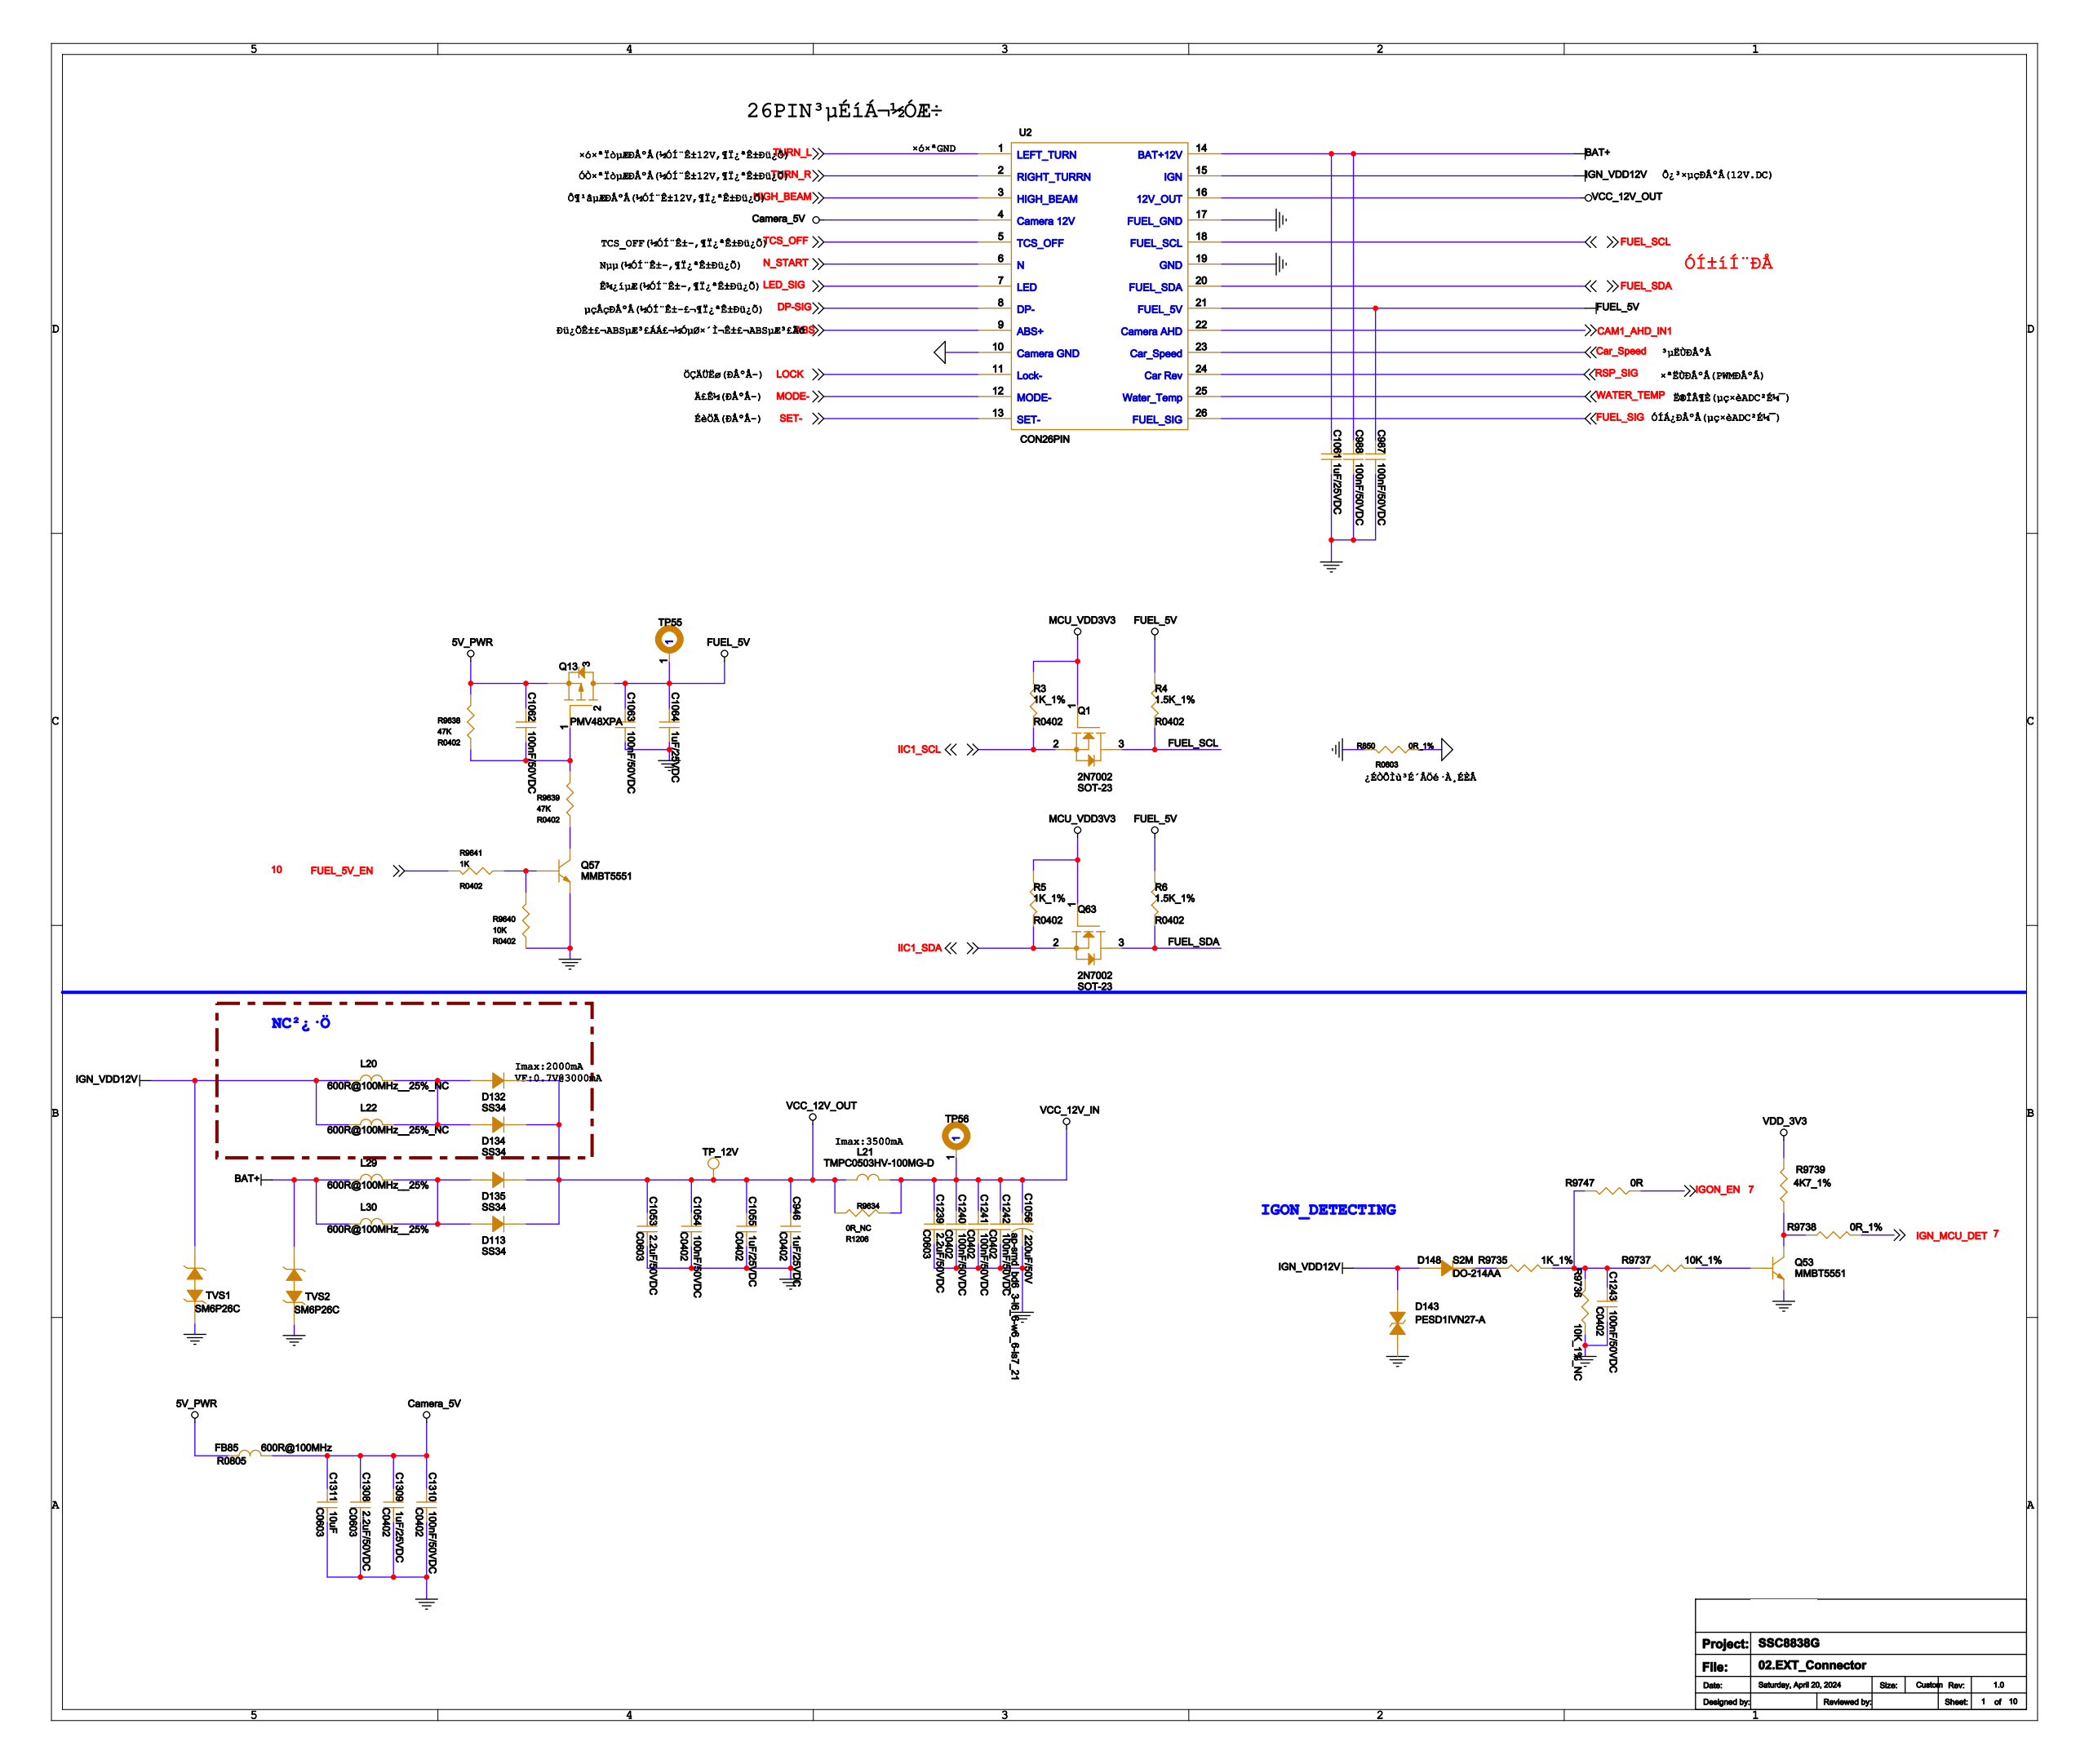Circuit board | Cadence Allegro | 958 parts | 601 nets | one sheet of the schematic
Parts on this sheet (reference | value | footprint):
C946 | 1uF/25VDC | C0402
C987 | 100nF/50VDC | C0402
C988 | 100nF/50VDC | C0402
C1053 | 2.2uF/50VDC | C0603
C1054 | 100nF/50VDC | C0402
C1055 | 1uF/25VDC | C0402
C1061 | 1uF/25VDC | C0402
C1062 | 100nF/50VDC | C0402
C1063 | 100nF/50VDC | C0402
C1064 | 1uF/25VDC | C0402
C1239 | 2.2uF/50VDC | C0603
C1240 | 100nF/50VDC | C0402
C1241 | 100nF/50VDC | C0402
C1242 | 100nF/50VDC | C0402
C1243 | 100nF/50VDC | C0402
C1308 | 2.2uF/50VDC | C0603
C1309 | 1uF/25VDC | C0402
C1310 | 100nF/50VDC | C0402
C1311 | 10uF | C0603
D113 | SS34 | SMB
D132 | SS34 | SMB
D134 | SS34 | SMB
D135 | SS34 | SMB
D143 | PESD1IVN27-A | SOD_323
D148 | S2M | DO-214AA
FB85 | 600R@100MHz | R0805
L20 | 600R@100MHz__25%_NC | R0805
L21 | TMPC0503HV-100MG-D | IND-5X5
L22 | 600R@100MHz__25%_NC | R0805
L29 | 600R@100MHz__25% | R0805
L30 | 600R@100MHz__25% | R0805
Q1 | 2N7002 | SOT-23
Q13 | PMV48XPA | SOT-23
Q53 | MMBT5551 | SOT-23
Q57 | MMBT5551 | SOT-23
Q63 | 2N7002 | SOT-23
R3 | 1K_1% | R0402
R4 | 1.5K_1% | R0402
R5 | 1K_1% | R0402
R6 | 1.5K_1% | R0402
R850 | 0R_1% | R0603
R9634 | 0R_NC | R1206
R9638 | 47K | R0402
R9639 | 47K | R0402
R9640 | 10K | R0402
R9641 | 1K | R0402
R9735 | 1K_1% | R0402
R9736 | 10K_1%_NC | R0402
R9737 | 10K_1% | R0402
R9738 | 0R_1% | R0402
R9739 | 4K7_1% | R0402
R9747 | 0R | R0402
TP55 | HOLE | TP_0R50
TP56 | HOLE | TP_0R50
TP_12V | Test_Point | TP_0R50
TVS1 | SM6P26C | DO214AB-A
TVS2 | SM6P26C | DO214AB-A
U2 | CON26PIN | CONN_26PIN_2_5MM_DIP
Nets of these parts (net: part-pin ...):
VCC_12V_IN: C1239-1 C1240-1 C1241-1 C1242-1 L21-2 R9634-2 TP56-1
GND: C946-2 C987-2 C988-2 C1053-2 C1054-2 C1055-2 C1061-2 C1063-2 C1064-2 C1239-2 C1240-2 C1241-2 C1242-2 C1243-2 C1308-2 C1309-2 C1310-2 C1311-2 D143-1 Q53-2 Q57-2 R850-2 R9640-1 R9736-1 TVS1-1 TVS2-1 U2-17 U2-19
5V_PWR: C1062-1 FB85-1 Q13-2 R9638-2
3V3_NORMAL: R9739-2
VCC_12V_OUT: C946-1 C1053-1 C1054-1 C1055-1 D113-2 D132-2 D134-2 D135-2 L21-1 R9634-1 TP_12V-1 U2-16
CAMERA_5V: C1308-1 C1309-1 C1310-1 C1311-1 FB85-2 U2-4
N21279287: C1062-2 Q13-1 R9638-1 R9639-2
FUEL_5V: C987-1 C1063-1 C1064-1 Q13-3 R4-1 R6-1 TP55-1 U2-21
N21387719: C1243-1 R9735-2 R9736-2 R9737-1 R9747-2
BAT+: C988-1 C1061-1 L29-1 L30-1 TVS2-2 U2-14
MCU_VDD3V3: Q1-1 Q63-1 R3-1 R5-1
N21253273: D113-1 D135-1 L29-2 L30-2
N21253247: D132-1 D134-1 L20-2 L22-2
DP-SIG: U2-8
IGN_VDD12V: D143-2 D148-1 L20-1 L22-1 TVS1-2 U2-15
LOCK: U2-11
ABS: U2-9
HIGH_BEAM: U2-3
TURN_R: U2-2
TURN_L: U2-1
TCS_OFF: U2-5
RSP_SIG: U2-24
LED_SIG: U2-7
FUEL_SIG: U2-26
WATER_TEMP: U2-25
N21387751: D148-2 R9735-1
IGON_EN: R9747-1
FUEL_SCL: Q1-3 R4-2 U2-18
IIC1_SCL: Q1-2 R3-2
FUEL_SDA: Q63-3 R6-2 U2-20
IIC1_SDA: Q63-2 R5-2
N21387737: Q53-1 R9737-2
N21387741: Q53-3 R9738-1 R9739-1
N21279333: Q57-1 R9640-2 R9641-1
N21279291: Q57-3 R9639-1
GND_SIGNAL: R850-1 U2-10
CAM1_AHD_IN1: U2-22
IGN_MCU_DET: R9738-2
FUEL_5V_EN: R9641-2